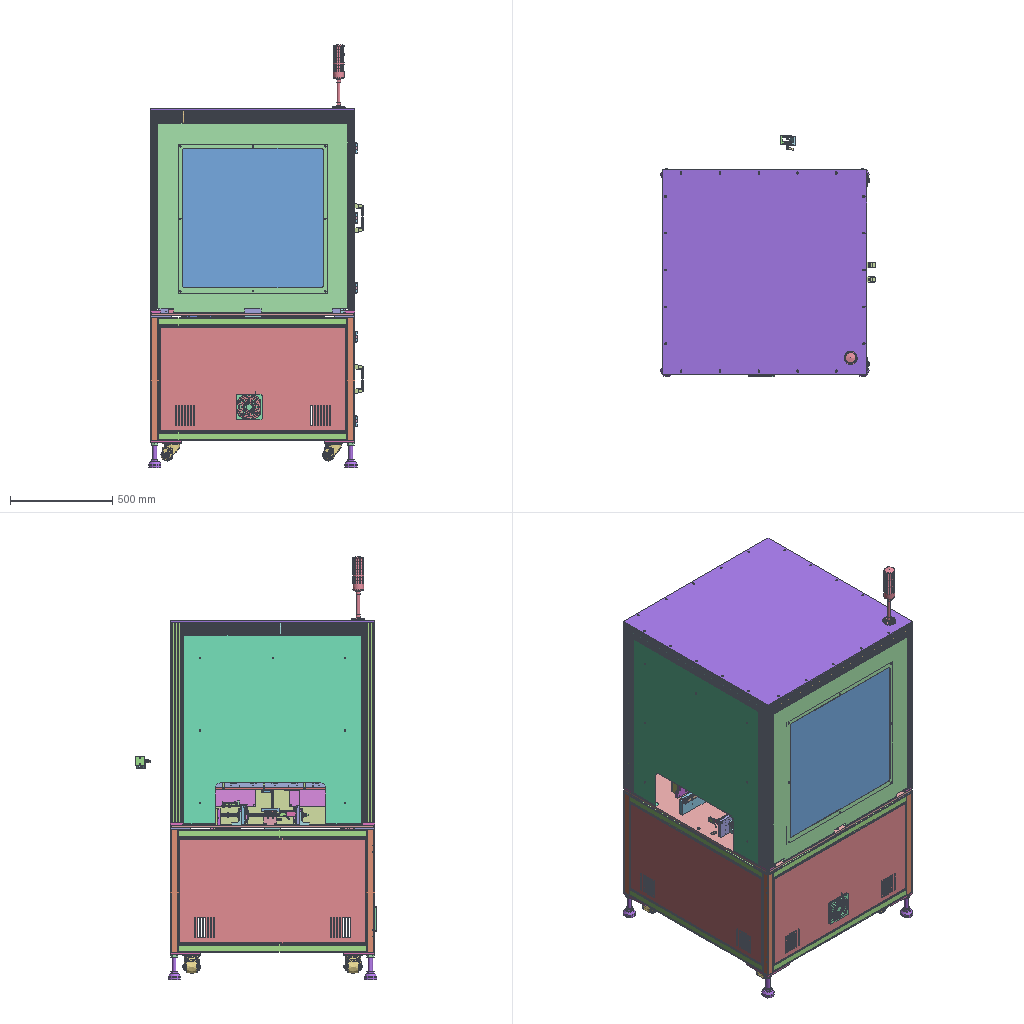Assembly | STEP file | 183 different items | 393 placed | box 1051 x 1181 x 2072 mm
Parts list (item | name | quantity | parent item | size | volume):
1 | 1-S938U-100524-003 | x1 | in Assembly-S938U-CTC-Long-Conveyor-Left | 95 x 915 x 15 mm | 1240006 mm3
2 | 1-S938U-100524-004 | x1 | in Assembly-S938U-CTC-Long-Conveyor-Right | 915 x 95 x 15 mm | 1230694 mm3
3 | 1-S938U-100524-006 | x8 | in Assembly-S938U-CTC-Long-Conveyor-Left, Assembly-S938U-CTC-Long-Conveyor-Right | 15 x 67 x 50 mm | 14485 mm3
4 | 1-S938U-100524-007 | x12 | in Assembly-S938U-CTC-Long-Conveyor-Left, Assembly-S938U-CTC-Long-Conveyor-Right | 12 x 12 x 23.5 mm | 1339 mm3
5 | 1-S938U-100524-008 | x12 | in Assembly-S938U-CTC-Long-Conveyor-Left, Assembly-S938U-CTC-Long-Conveyor-Right | 12 x 12 x 2 mm | 169.646 mm3
6 | 1-S938U-100524-009 | x12 | in Assembly-S938U-CTC-Long-Conveyor-Bearing | 10 x 10 x 1 mm | 50.265 mm3
7 | 1-S938U-100524-012 | x1 | in Assembly-S938U-CTC-Long-Conveyor | 170 x 60 x 75 mm | 13658 mm3
8 | BODY10_E-RAM6-S-640-ME30-C5 | x2 | in E-RAM6-S-640-ME30-C5 | 40 x 4.5 x 795.5 mm | 67309 mm3
9 | BODY1_E-RAM6-S-640-ME30-C5 | x2 | in E-RAM6-S-640-ME30-C5 | 63 x 51 x 780 mm | 1225538 mm3
10 | BODY22_E-RAM6-S-640-ME30-C5 | x2 | in E-RAM6-S-640-ME30-C5 | 720 x 10 x 1.5 mm | 10800 mm3
11 | BODY2_E-RAM6-S-640-ME30-C5 | x2 | in E-RAM6-S-640-ME30-C5 | 29.5 x 14 x 759.7 mm | 139980 mm3
12 | BODY3_E-RAM6-S-640-ME30-C5 | x4 | in E-RAM6-S-640-ME30-C5 | 5 x 3 x 780 mm | 9747 mm3
13 | BODY4_E-RAM6-S-640-ME30-C5 | x4 | in E-RAM6-S-640-ME30-C5 | 60 x 64.65 x 22 mm | 24939 mm3
14 | BODY5_E-RAM6-S-640-ME30-C5 | x2 | in E-RAM6-S-640-ME30-C5 | 74.25 x 45.4 x 96 mm | 131953 mm3
15 | BODY6_E-RAM6-S-640-ME30-C5 | x4 | in E-RAM6-S-640-ME30-C5 | 34.8 x 15.5 x 3.15 mm | 724.972 mm3
16 | BODY7_E-RAM6-S-640-ME30-C5 | x2 | in E-RAM6-S-640-ME30-C5 | 20.3 x 33.5 x 56 mm | 16364 mm3
17 | BODY8_E-RAM6-S-640-ME30-C5 | x4 | in E-RAM6-S-640-ME30-C5 | 14.5 x 43.5 x 12 mm | 744.799 mm3
18 | BODY9_E-RAM6-S-640-ME30-C5 | x6 | in E-RAM6-S-640-ME30-C5 | 25.93 x 28.65 x 17.21 mm | 1817 mm3
19 | BODYDZ_E-RAM6-S-640-ME30-C5 | x1 | in MOVERS_E-RAM6-S-640-ME30-C5 | 31.85 x 18 x 222.5 mm | 8435 mm3
20 | BODYMSM_E-RAM6-S-640-ME30-C5 | x1 | in MOVERS_E-RAM6-S-640-ME30-C5 | 14.9 x 31.1 x 221.16 mm | 25998 mm3
21 | BOLT3-8 | x4 | in C-KSC5010-B1-300-F1 | 11 x 5.5 x 5.5 mm | 117.995 mm3
22 | BOLT4-12 | x8 | in LX4520CP-MX-B1-A4560-590-EP3 | 16 x 7 x 7 mm | 285.431 mm3
23 | Basler ace 2 USB3-1-1-1 | x1 | in ASS CHECK TAPE | 3.68 x 1.85 x 1.85 mm | 2.495 mm3
24 | Basler ace 2 USB3-1-1-1_1 | x1 | in ASS CHECK TAPE | 3.68 x 1.85 x 1.85 mm | 2.495 mm3
25 | Basler ace 2 USB3-1-1-1_10 | x1 | in ASS CHECK TAPE | 1.96 x 0.2 x 1.96 mm | 0.2322 mm3
26 | Basler ace 2 USB3-1-1-1_12 | x1 | in ASS CHECK TAPE | 0.85 x 5.522 x 4.3 mm | 2.553 mm3
27 | Basler ace 2 USB3-1-1-1_2 | x1 | in ASS CHECK TAPE | 0.85 x 5.522 x 4.3 mm | 2.556 mm3
28 | Basler ace 2 USB3-1-1-1_3 | x1 | in ASS CHECK TAPE | 3.68 x 1.85 x 1.85 mm | 2.494 mm3
29 | Basler ace 2 USB3-1-1-1_4 | x1 | in ASS CHECK TAPE | 3.68 x 1.85 x 1.85 mm | 2.494 mm3
30 | Basler ace 2 USB3-1-1-1_5 | x1 | in ASS CHECK TAPE | 1.96 x 0.2 x 1.96 mm | 0.2322 mm3
31 | Basler ace 2 USB3-1-1-1_8 | x1 | in ASS CHECK TAPE | 3.68 x 1.85 x 1.85 mm | 2.495 mm3
32 | Basler ace 2 USB3-1-1-1_9 | x1 | in ASS CHECK TAPE | 3.68 x 1.85 x 1.85 mm | 2.495 mm3
33 | Basler ace USB3 C-Mount v02-1-1_17 | x1 | in ASS CHECK TAPE | 29 x 29 x 48.2 mm | 25313 mm3
34 | C-CFJFNV60-20-150_b | x4 | in C-CFJFNV60-20-150 | 190.5 x 60 x 60 mm | 129714 mm3
35 | C-CFJFNV60-20-150_n | x4 | in C-CFJFNV60-20-150 | 16 x 34.641 x 30 mm | 8537 mm3
36 | C-HHFLS6-5 | x10 | in Assembly-Fix Bot Cover, Assembly-Fix-TheDoor1 | 44 x 53.4 x 11.5 mm | 9579 mm3
37 | C-HLGHA20-850_r | x1 | in C-HLGHA20-850 | 20 x 17.5 x 850 mm | 242038 mm3
38 | C-HLGHAB20 | x1 | in C-HLGHA20-850 | 44 x 25.4 x 108.25 mm | 81548 mm3
39 | C-HTPA20S5M100-A-N10 | x1 | in Assembly-S938U-CTC-Long-Conveyor-Motor | 16 x 36 x 36 mm | 9752 mm3
40 | C-KS50-300_c | x1 | in C-KSC5010-B1-300-F1 | 320 x 5 x 45 mm | 26928 mm3
41 | C-KS50-F1_ma | x1 | in C-KSC5010-B1-300-F1 | 10.5 x 40 x 40 mm | 8273 mm3
42 | C-KSC50-B1-1-NS_bl | x1 | in C-KSC5010-B1-300-F1 | 76 x 30.8 x 62 mm | 62545 mm3
43 | C-KSC5010-B1-300-F1_b | x1 | in C-KSC5010-B1-300-F1 | 370 x 38.5 x 50 mm | 223115 mm3
44 | C-MPU20-40-38-26-S20-9 | x2 | in Assembly-Fix-XYZR | - | 259932 mm3
45 | CLDMC4-12-M | x9 | in Assembly-Fix-XYZR | 36.5 x 41 x 13 mm | 4938 mm3
46 | CST-2BS14738W-1-1-11111 | x2 | in Assembly-Fix-light | 27.023 x 150 x 38 mm | 125802 mm3
47 | E-1238D24-SRF | x1 | in Assembly-Fix-Body | 120 x 135 x 38 mm | 131413 mm3
48 | E-MSM320RYG-C | x1 | in Assembly-Fix Top Cover Big | 65 x 314 x 64.82 mm | 382471 mm3
49 | E-PF-120-R | x1 | in Assembly-Fix-Body | 125 x 10 x 125 mm | 66671 mm3
50 | E-SFG-120-R | x1 | in Assembly-Fix-Body | 115 x 5 x 115 mm | 4127 mm3
51 | FB10-16_ | x1 | in SH-HBLTBBN45 | 16 x 20 x 20 mm | 1741 mm3
52 | FB10-16_ [2] | x1 | in SL-HBLTBBN45 | 16 x 20 x 20 mm | 1741 mm3
53 | GCJS20-RD-5-8 | x1 | in Assembly-Fix-XYZR | 30 x 20 x 20 mm | 8182 mm3
54 | GLH-60-ASF | x4 | in Assembly-Fix Bot Cover | 100 x 90 x 92 mm | 321084 mm3
55 | HBLTBBN45_b | x1 | in SH-HBLTBBN45 | 55 x 45 x 45 mm | 44256 mm3
56 | HBLTBBN45_b [2] | x1 | in SL-HBLTBBN45 | 55 x 45 x 45 mm | 44256 mm3
57 | LX4520CP-MX-B1-590-EP3-ASL_bl | x2 | in LX4520CP-MX-B1-A4560-590-EP3 | 104 x 45 x 137.6 mm | 272574 mm3
58 | LX4520CP-MX-B1-590-EP3_f | x2 | in LX4520CP-MX-B1-A4560-590-EP3 | 22 x 17.4 x 9.4 mm | 629.359 mm3
59 | LX4520CP-MX-B1-590_c | x2 | in LX4520CP-MX-B1-A4560-590-EP3 | 77 x 6.5 x 615 mm | 143031 mm3
60 | LX4520CP-MX-B1-A4560-590-EP3_b | x2 | in LX4520CP-MX-B1-A4560-590-EP3 | 677 x 56 x 80 mm | 1131929 mm3
61 | LX_SENSOR_SET-EP | x6 | in LX4520CP-MX-B1-A4560-590-EP3 | 27.925 x 13.5 x 21.3 mm | 2192 mm3
62 | ME30_E-RAM6-S-640-ME30-C5 | x1 | in MOVERS_E-RAM6-S-640-ME30-C5 | 155.627 x 153.2 x 43 mm | 932829 mm3
63 | P0278200003_D | x1 | in AH064_2ST_8_ASM | 34.5 x 88 x 88 mm | 90794 mm3
64 | P0359210003_D | x1 | in AH064_2ST_8_ASM | 15 x 40 x 40 mm | 15757 mm3
65 | P0409101803-0002 | x1 | in AH064_2ST_8-P0409101803 | 70 x 70 x 21.5 mm | 78366 mm3
66 | P0503100005_D | x1 | in AH064_2ST_8_ASM | 13 x 29.5 x 29.481 mm | 6728 mm3
67 | P0912100001_D | x1 | in AH064_2ST_8_ASM | 36.5 x 17 x 17 mm | 4717 mm3
68 | P1211200001_D | x1 | in AH064_2ST_8_ASM | 49.654 x 7 x 49.654 mm | 6705 mm3
69 | P1317200001_D | x1 | in AH064_2ST_8_ASM | 45.5 x 76 x 76 mm | 152294 mm3
70 | ROTATION MC_NEW VER-0610_1014 | x1 | in Assembly-S938U-CTC-Long-Conveyor-Left | 32 x 7 x 32 mm | 3384 mm3
71 | ROTATION MC_NEW VER-0610_1015 | x1 | in Assembly-S938U-CTC-Long-Conveyor-Left | 32 x 7 x 32 mm | 3384 mm3
72 | ROTATION MC_NEW VER-0610_1017 | x1 | in Assembly-S938U-CTC-Long-Conveyor-Left | 44 x 51.28 x 44 mm | 22323 mm3
73 | ROTATION MC_NEW VER-0610_1018 | x1 | in Assembly-S938U-CTC-Long-Conveyor-Right | 32 x 7 x 32 mm | 3384 mm3
74 | ROTATION MC_NEW VER-0610_1019 | x1 | in Assembly-S938U-CTC-Long-Conveyor | 23.05 x 1.2 x 25.6 mm | 179.471 mm3
75 | ROTATION MC_NEW VER-0610_1020 | x1 | in Assembly-S938U-CTC-Long-Conveyor-Right | 32 x 7 x 32 mm | 3384 mm3
76 | ROTATION MC_NEW VER-0610_1021 | x2 | in Assembly-S938U-CTC-Long-Conveyor-Left, Assembly-S938U-CTC-Long-Conveyor-Right | 63 x 32 x 67 mm | 57913 mm3
77 | ROTATION MC_NEW VER-0610_1022 | x1 | in Assembly-S938U-CTC-Long-Conveyor-Right | 44 x 51.28 x 44 mm | 22323 mm3
78 | ROTATION MC_NEW VER-0610_472 | x1 | in Assembly-S938U-CTC-Long-Conveyor-Cylinder keep | 4.4 x 40.5 x 5.8 mm | 628.814 mm3
79 | ROTATION MC_NEW VER-0610_473 | x1 | in Assembly-S938U-CTC-Long-Conveyor-Cylinder keep | 4.4 x 40.5 x 5.8 mm | 628.814 mm3
80 | ROTATION MC_NEW VER-0610_474 | x1 | in Assembly-S938U-CTC-Long-Conveyor-Cylinder keep | 44 x 74.1 x 15 mm | 10477 mm3
81 | ROTATION MC_NEW VER-0610_475 | x1 | in Assembly-S938U-CTC-Long-Conveyor-Cylinder keep | 46 x 74 x 17 mm | 39831 mm3
82 | ROTATION MC_NEW VER-0610_476 | x1 | in Assembly-S938U-CTC-Long-Conveyor | 3 x 4 x 4 mm | 27.73 mm3
83 | ROTATION MC_NEW VER-0610_477 | x1 | in Assembly-S938U-CTC-Long-Conveyor-Motor | 36 x 16 x 36 mm | 10187 mm3
84 | ROTATION MC_NEW VER-0610_478 | x1 | in Assembly-S938U-CTC-Long-Conveyor | 4.306 x 4 x 4.085 mm | 27.73 mm3
85 | ROTATION MC_NEW VER-0610_479 | x1 | in Assembly-S938U-CTC-Long-Conveyor-Right | 32 x 7 x 32 mm | 3384 mm3
86 | ROTATION MC_NEW VER-0610_486 | x1 | in Assembly-S938U-CTC-Long-Conveyor | 14.5 x 5.5 x 14.5 mm | 476.246 mm3
87 | ROTATION MC_NEW VER-0610_487 | x1 | in Assembly-S938U-CTC-Long-Conveyor | 14.5 x 5.5 x 14.5 mm | 476.246 mm3
88 | ROTATION MC_NEW VER-0610_488 | x1 | in Assembly-S938U-CTC-Long-Conveyor | 16 x 8 x 16 mm | 1383 mm3
89 | ROTATION MC_NEW VER-0610_489 | x1 | in Assembly-S938U-CTC-Long-Conveyor | 42 x 27 x 42 mm | 26913 mm3
90 | ROTATION MC_NEW VER-0610_494 | x1 | in Assembly-S938U-CTC-Long-Conveyor-Cylinder-1 | 26 x 58 x 49 mm | 47669 mm3
91 | ROTATION MC_NEW VER-0610_495 | x1 | in Assembly-S938U-CTC-Long-Conveyor-Cylinder-1 | 22 x 56 x 57.5 mm | 14884 mm3
92 | ROTATION MC_NEW VER-0610_496 | x1 | in Assembly-S938U-CTC-Long-Conveyor-Cylinder-1 | 8.083 x 5.5 x 7 mm | 161.093 mm3
93 | ROTATION MC_NEW VER-0610_497 | x1 | in Assembly-S938U-CTC-Long-Conveyor-Cylinder-1 | 8.083 x 5.5 x 7 mm | 161.093 mm3
94 | ROTATION MC_NEW VER-0610_498 | x1 | in Assembly-S938U-CTC-Long-Conveyor-Cylinder-1 | 4.6 x 4 x 36 mm | 360.691 mm3
95 | ROTATION MC_NEW VER-0610_499 | x1 | in Assembly-S938U-CTC-Long-Conveyor-Cylinder-1 | 4.6 x 4 x 36 mm | 360.69 mm3
96 | ROTATION MC_NEW VER-0610_500 | x1 | in Assembly-S938U-CTC-Long-Conveyor-Cylinder-2 | 26 x 58 x 49 mm | 47669 mm3
97 | ROTATION MC_NEW VER-0610_501 | x1 | in Assembly-S938U-CTC-Long-Conveyor-Cylinder-2 | 22 x 56 x 57.5 mm | 14884 mm3
98 | ROTATION MC_NEW VER-0610_502 | x1 | in Assembly-S938U-CTC-Long-Conveyor-Cylinder-2 | 8.083 x 5.5 x 7 mm | 161.093 mm3
99 | ROTATION MC_NEW VER-0610_503 | x1 | in Assembly-S938U-CTC-Long-Conveyor-Cylinder-2 | 8.083 x 5.5 x 7 mm | 161.093 mm3
100 | ROTATION MC_NEW VER-0610_504 | x1 | in Assembly-S938U-CTC-Long-Conveyor-Cylinder-2 | 4.6 x 4 x 36 mm | 360.691 mm3
101 | ROTATION MC_NEW VER-0610_505 | x1 | in Assembly-S938U-CTC-Long-Conveyor-Cylinder-2 | 4.6 x 4 x 36 mm | 360.69 mm3
102 | ROTATION MC_NEW VER-0610_507 | x3 | in Assembly-S938U-CTC-Long-Conveyor-Sensor | 11 x 48.371 x 37.42 mm | 6844 mm3
103 | ROTATION MC_NEW VER-0610_516 | x3 | in Assembly-S938U-CTC-Long-Conveyor-Sensor | 41.5 x 81.002 x 21 mm | 3574 mm3
104 | ROTATION MC_NEW VER-0610_519 | x12 | in Assembly-S938U-CTC-Long-Conveyor-Bearing | 19 x 6 x 19 mm | 1113 mm3
105 | ROTATION MC_NEW VER-0610_532 | x12 | in Assembly-S938U-CTC-Long-Conveyor-Bearing | 19 x 6 x 19 mm | 1113 mm3
106 | ROTATION MC_NEW VER-0610_539 | x1 | in Assembly-S938U-CTC-Long-Conveyor-Cylinder keep | 51 x 8 x 51 mm | 17634 mm3
107 | ROTATION MC_NEW VER-0610_540 | x1 | in Assembly-S938U-CTC-Long-Conveyor-Cylinder keep | 51 x 99 x 11 mm | 28554 mm3
108 | ROTATION MC_NEW VER-0610_541 | x1 | in Assembly-S938U-CTC-Long-Conveyor | 12 x 481.5 x 13.856 mm | 56212 mm3
109 | ROTATION MC_NEW VER-0610_543 | x1 | in Assembly-S938U-CTC-Long-Conveyor-Cylinder-2 | 24 x 30 x 10 mm | 1863 mm3
110 | ROTATION MC_NEW VER-0610_544 | x1 | in Assembly-S938U-CTC-Long-Conveyor-Cylinder-2 | 24 x 30 x 10 mm | 1863 mm3
111 | ROTATION MC_NEW VER-0610_545 | x1 | in Assembly-S938U-CTC-Long-Conveyor-Cylinder keep | 30 x 10 x 24 mm | 1863 mm3
112 | ROTATION MC_NEW VER-0610_546 | x1 | in Assembly-S938U-CTC-Long-Conveyor-Cylinder-1 | 24 x 30 x 10 mm | 1863 mm3
113 | ROTATION MC_NEW VER-0610_547 | x1 | in Assembly-S938U-CTC-Long-Conveyor-Cylinder-1 | 24 x 30 x 10 mm | 1863 mm3
114 | ROTATION MC_NEW VER-0610_548 | x1 | in Assembly-S938U-CTC-Long-Conveyor-Cylinder keep | 30 x 10 x 24 mm | 1863 mm3
115 | ROTATION MC_NEW VER-0610_549 | x1 | in Assembly-S938U-CTC-Long-Conveyor-Cylinder-2 | 48 x 64 x 12 mm | 35212 mm3
116 | ROTATION MC_NEW VER-0610_550 | x1 | in Assembly-S938U-CTC-Long-Conveyor-Cylinder-1 | 48 x 64 x 12 mm | 35212 mm3
117 | ROTATION MC_NEW VER-0610_551 | x1 | in Assembly-S938U-CTC-Long-Conveyor-Cylinder-2 | 10 x 64 x 63 mm | 38849 mm3
118 | ROTATION MC_NEW VER-0610_552 | x1 | in Assembly-S938U-CTC-Long-Conveyor-Cylinder-1 | 10 x 64 x 63 mm | 38849 mm3
119 | ROTATION MC_NEW VER-0610_553 | x1 | in Assembly-S938U-CTC-Long-Conveyor-Cylinder-2 | 46 x 90 x 15 mm | 41116 mm3
120 | ROTATION MC_NEW VER-0610_554 | x1 | in Assembly-S938U-CTC-Long-Conveyor-Cylinder-1 | 46 x 90 x 15 mm | 41116 mm3
121 | ROTATION MC_NEW VER-0610_555 | x1 | in Assembly-S938U-CTC-Long-Conveyor-Cylinder keep | 54 x 47.54 x 24.76 mm | 18101 mm3
122 | ROTATION MC_NEW VER-0610_564 | x1 | in Assembly-S938U-CTC-Long-Conveyor-Motor | 10 x 120 x 95.441 mm | 51150 mm3
123 | ROTATION MC_NEW VER-0610_565 | x1 | in Assembly-S938U-CTC-Long-Conveyor-Motor | 10 x 120 x 95.441 mm | 51150 mm3
124 | ROTATION MC_NEW VER-0610_566 | x1 | in Assembly-S938U-CTC-Long-Conveyor | 10 x 43 x 80 mm | 22787 mm3
125 | ROTATION MC_NEW VER-0610_568 | x1 | in Assembly-S938U-CTC-Long-Conveyor | 10 x 43 x 80 mm | 22787 mm3
126 | ROTATION MC_NEW VER-0610_572 | x1 | in Assembly-S938U-CTC-Long-Conveyor | 154.5 x 43.5 x 81.5 mm | 37915 mm3
127 | ROTATION MC_NEW VER-0610_577 | x1 | in Assembly-S938U-CTC-Long-Conveyor | 204 x 15 x 80 mm | 192729 mm3
128 | ROTATION MC_NEW VER-0610_578 | x1 | in Assembly-S938U-CTC-Long-Conveyor-Right | 867 x 12.8 x 16 mm | 173749 mm3
129 | ROTATION MC_NEW VER-0610_579 | x1 | in Assembly-S938U-CTC-Long-Conveyor-Left | 867 x 12.8 x 16 mm | 173749 mm3
130 | ROTATION MC_NEW VER-0610_582 | x2 | in Assembly-S938U-CTC-Long-Conveyor-Left, Assembly-S938U-CTC-Long-Conveyor-Right | 910.4 x 10 x 79.4 mm | 24385 mm3
131 | ROTATION MC_NEW VER-0610_583 | x1 | in Assembly-S938U-CTC-Long-Conveyor-Motor | 58.82 x 10 x 151.249 mm | 5398 mm3
132 | ROTATION MC_NEW VER-0610_980 | x1 | in Assembly-S938U-CTC-Long-Conveyor-Motor | 114 x 10 x 100 mm | 101269 mm3
133 | ROTATION MC_NEW VER-0610_981 | x1 | in Assembly-S938U-CTC-Long-Conveyor-Motor | 141 x 18 x 139 mm | 139534 mm3
134 | S7I15G_T | x1 | in Assembly-S938U-CTC-Long-Conveyor-Motor | 93.4 x 99.5 x 70 mm | 343448 mm3
135 | S7KA3-18 | x1 | in Assembly-S938U-CTC-Long-Conveyor-Motor | 70 x 70 x 64 mm | 137824 mm3
136 | SCB3-6 | x12 | in LX4520CP-MX-B1-A4560-590-EP3 | 9 x 5.5 x 5.5 mm | 103.858 mm3
137 | SENC3-600-LX45-590_lx | x2 | in LX4520CP-MX-B1-A4560-590-EP3 | 600 x 19 x 6 mm | 30746 mm3
138 | SynoNew-0304-024 | x6 | in Assembly-Fix Bot Cover, Assembly-Fix-chan | 120 x 100 x 12 mm | 109561 mm3
139 | SynoNew-0304-025 | x1 | - | 1000 x 1000 x 12 mm | 11833739 mm3
140 | SynoNew-0304-026 | x1 | in Assembly-Fix-XYZR | 100 x 802 x 10 mm | 789361 mm3
141 | SynoNew-0304-027 | x1 | in Assembly-Fix-XYZR | 100 x 912 x 10 mm | 899646 mm3
142 | SynoNew-0304-028 | x1 | in Assembly-Fix-XYZR | 65 x 800 x 8 mm | 354237 mm3
143 | SynoNew-0304-029 | x5 | in Assembly-Fix-XYZR | 185 x 113 x 8 mm | 35447 mm3
144 | SynoNew-0304-030 | x1 | in Assembly-Fix-XYZR | 50 x 850 x 10 mm | 419787 mm3
145 | SynoNew-0304-031 | x1 | in Assembly-Fix-XYZR | 50 x 93.3 x 20 mm | 69168 mm3
146 | SynoNew-0304-032 | x3 | in Assembly-Fix-XYZR | 15 x 120 x 50 mm | 51097 mm3
147 | SynoNew-0304-033 | x1 | in Assembly-Fix-XYZR | 185 x 96 x 10 mm | 142101 mm3
148 | SynoNew-0304-038 | x1 | in Assembly-Fix-XYZR | 210 x 70 x 10 mm | 117309 mm3
149 | SynoNew-0304-039 | x1 | in Assembly-Fix-XYZR | 100 x 280 x 8 mm | 182196 mm3
150 | SynoNew-0304-040 | x1 | in Assembly-Fix-XYZR | 100 x 160 x 8 mm | 111423 mm3
151 | SynoNew-0304-041 | x4 | in Assembly-Fix Bot Cover | 40 x 600 x 40 mm | 266067 mm3
152 | SynoNew-0304-042 | x4 | in Assembly-Fix Bot Cover | 100 x 100 x 10 mm | 99668 mm3
153 | SynoNew-0304-043 | x10 | in Assembly-Fix Bot Cover | 40 x 920 x 40 mm | 408480 mm3
154 | SynoNew-0304-044 | x4 | in Assembly-Fix Bot Cover | 150 x 150 x 10 mm | 221263 mm3
155 | SynoNew-0304-045 | x4 | in Assembly-Fix Bot Cover | 40 x 80 x 10 mm | 31668 mm3
156 | SynoNew-0304-046 | x4 | in Assembly-Fix-light | 60 x 40 x 28 mm | 9653 mm3
157 | SynoNew-0304-047 | x1 | in Assembly-Fix-XYZR | 100 x 160 x 8 mm | 111423 mm3
158 | SynoNew-0304-048 | x4 | in Assembly-Fix Top Cover | 60 x 30 x 980 mm | 587031 mm3
159 | SynoNew-0304-049 | x4 | in Assembly-Fix Top Cover | 60 x 50 x 12 mm | 33116 mm3
160 | SynoNew-0304-050 | x2 | in Assembly-Fix Top Cover Big | 60 x 30 x 880 mm | 527129 mm3
161 | SynoNew-0304-051 | x2 | in Assembly-Fix Top Cover Big | 60 x 30 x 940 mm | 563070 mm3
162 | SynoNew-0304-052 | x3 | in Assembly-Fix Bot Cover | 515 x 915 x 25 mm | 790603 mm3
163 | SynoNew-0304-053 | x2 | in Assembly-Fix Bot Cover | 515 x 457 x 25 mm | 405617 mm3
164 | SynoNew-0304-054 | x1 | in Assembly-Fix-XYZR | 890 x 70 x 1.5 mm | 89689 mm3
165 | SynoNew-0304-055 | x1 | in Assembly-Fix Top Cover Big | 1000 x 1000 x 10 mm | 9984549 mm3
166 | SynoNew-0304-056 | x2 | in Assembly-Fix-XYZR | 40 x 80 x 2 mm | 3100 mm3
167 | SynoNew-0304-057 | x2 | in Assembly-Fix Top Cover Big | 928 x 936 x 25 mm | 704183 mm3
168 | SynoNew-0304-058 | x1 | in Assembly-Fix Bot Cover | 945 x 945 x 3 mm | 2628455 mm3
169 | SynoNew-0304-059 | x2 | in Assembly-Fix Top Cover Big | 730 x 730 x 10 mm | 5327429 mm3
170 | SynoNew-0304-060 | x2 | in Assembly-Fix-TheDoor1 | 437 x 930 x 25 mm | 451749 mm3
171 | SynoNew-0304-061 | x2 | in Assembly-Fix-TheDoor1 | 277 x 750 x 10 mm | 2076322 mm3
172 | SynoNew-0304-062 | x5 | in Assembly-Fix-XYZR | 6 x 6 x 20 mm | 551.703 mm3
173 | SynoNew-0304-063 | x1 | in Assembly-Fix-XYZR | 802 x 100 x 60 mm | 195750 mm3
174 | SynoNew-0304-064 | x1 | in Assembly-Fix-XYZR | 258 x 120 x 45 mm | 48671 mm3
175 | SynoNew-0304-065 | x1 | in ASS CHECK TAPE | 100 x 12 x 100 mm | 87539 mm3
176 | SynoNew-0304-066 | x1 | in ASS CHECK TAPE | 60 x 10 x 55 mm | 13958 mm3
177 | SynoNew-0304-067 | x1 | in ASS CHECK TAPE | 60 x 10 x 10 mm | 4574 mm3
178 | SynoNew-0304-068 | x1 | in Assembly-Fix Bot Cover | 500 x 350 x 30 mm | 283151 mm3
179 | SynoNew-0304-069 | x1 | in Assembly-Fix Top Cover Big | 928 x 876 x 25 mm | 1155671 mm3
180 | UPCN26-M-41-SET | x4 | in Assembly-Fix Bot Cover, Assembly-Fix-TheDoor1 | 139 x 52.5 x 26 mm | 44539 mm3
181 | VS-TEV0305-1-1-1 | x1 | in ASS CHECK TAPE | 111.97 x 59.35 x 55 mm | 201567 mm3
182 | hg-kr13_ | x2 | in Assembly-Fix-XYZR | 41.2 x 49.5 x 107.4 mm | 131615 mm3
183 | lx4510_A4560 | x2 | in LX4520CP-MX-B1-A4560-590-EP3 | 62 x 60 x 10 mm | 18303 mm3